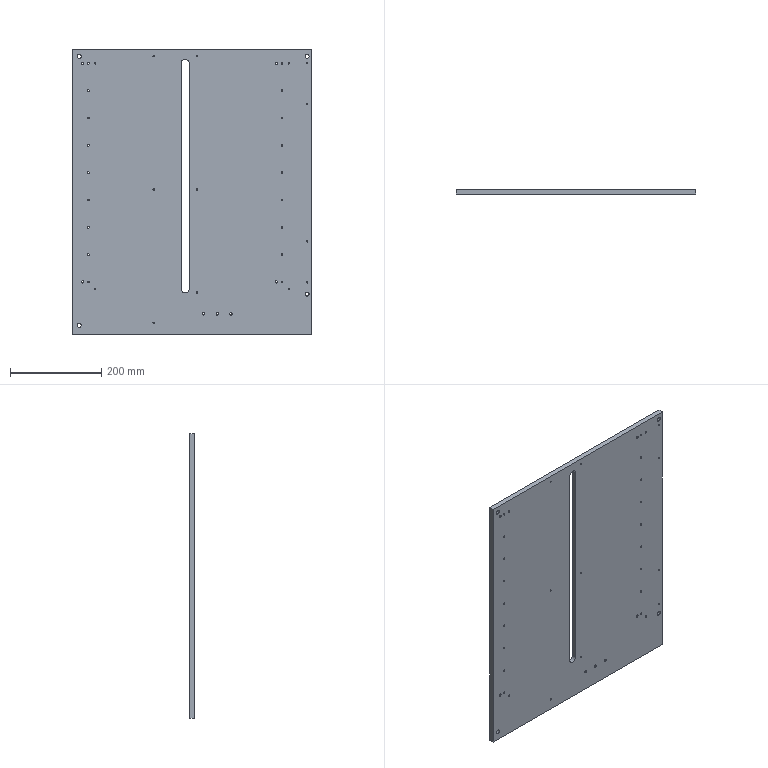Part | STEP file | 0243_202_Plate | 1 solid | 97 faces | box 525 x 10 x 625 mm | volume 3182017 mm3 | cylinder 89 | plane 8 | commonest cylinder face diameters 4.2 x36 3.3 x20 2.5 x8 5 x8 9 x8 5.5 x6